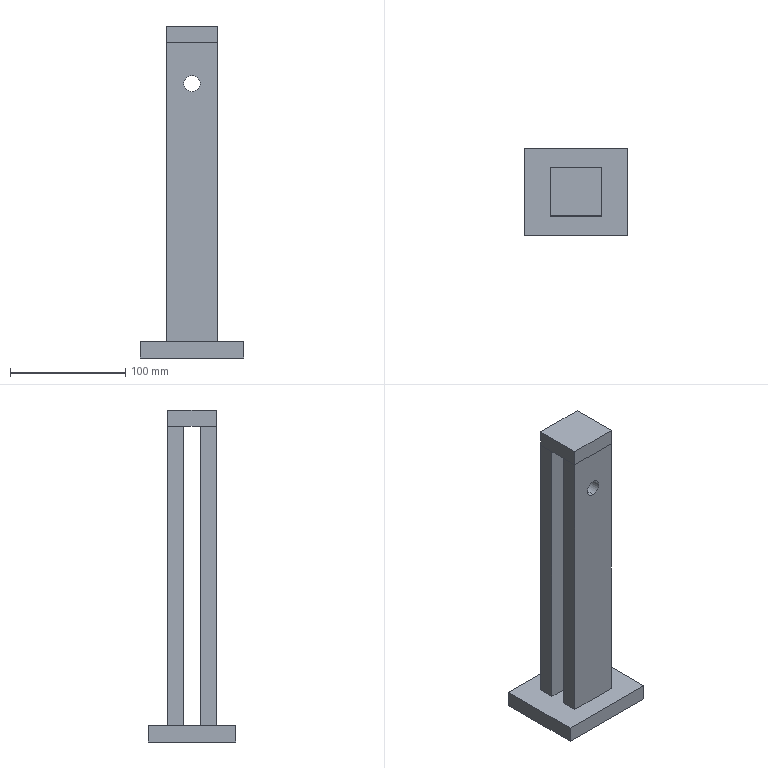Part | STEP file | Backup 2012-3-22-019 | 1 solid | 26 faces | box 90 x 76 x 288 mm | volume 445485 mm3 | plane 22 | cylinder 4 | commonest cylinder face diameters 14 x4